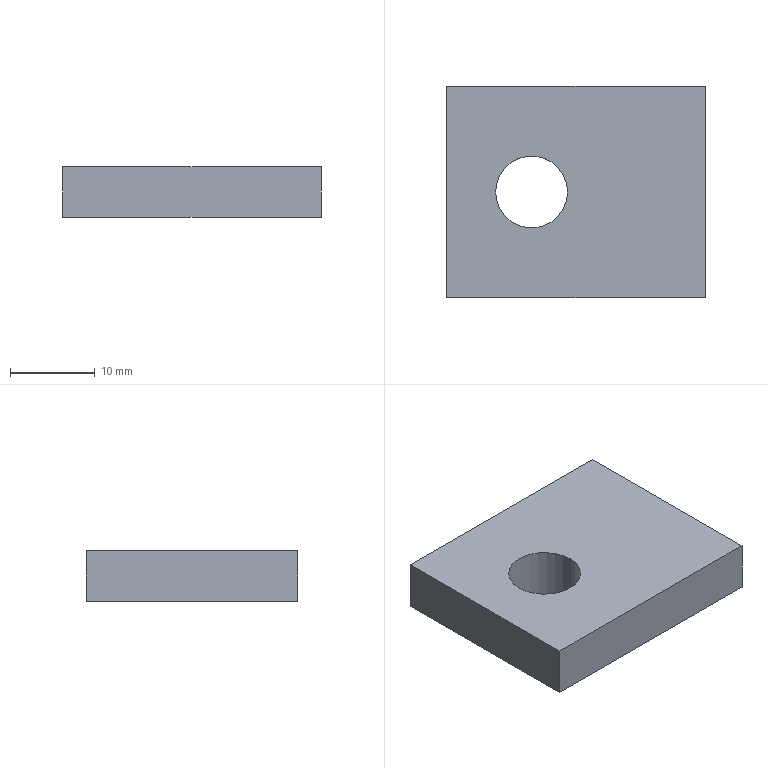Part | SolidWorks | features Extrusion 1 | 1 solid | 8 faces | box 30.5 x 25 x 6 mm | volume 4235 mm3 | plane 6 | cylinder 2 | commonest cylinder face diameters 8.5 x2
STEP:
#1=CARTESIAN_POINT('',(-30.85,-55.606,6.));
#2=VERTEX_POINT('',#1);
#3=CARTESIAN_POINT('',(-22.35,-55.606,6.));
#4=VERTEX_POINT('',#3);
#5=CARTESIAN_POINT('',(-26.6,-55.606,6.));
#6=DIRECTION('',(0.,0.,1.));
#7=DIRECTION('',(1.,0.,0.));
#8=AXIS2_PLACEMENT_3D('',#5,#6,#7);
#9=CIRCLE('',#8,4.25);
#10=EDGE_CURVE('',#2,#4,#9,.T.);
#11=ORIENTED_EDGE('',*,*,#10,.T.);
#12=CARTESIAN_POINT('',(-22.35,-55.606,0.));
#13=VERTEX_POINT('',#12);
#14=CARTESIAN_POINT('',(-22.35,-55.606,6.));
#15=DIRECTION('',(0.,0.,-1.));
#16=VECTOR('',#15,1000.);
#17=LINE('',#14,#16);
#18=EDGE_CURVE('',#4,#13,#17,.T.);
#19=ORIENTED_EDGE('',*,*,#18,.T.);
#20=CARTESIAN_POINT('',(-30.85,-55.606,0.));
#21=VERTEX_POINT('',#20);
#22=CARTESIAN_POINT('',(-26.6,-55.606,0.));
#23=DIRECTION('',(0.,0.,1.));
#24=DIRECTION('',(1.,0.,0.));
#25=AXIS2_PLACEMENT_3D('',#22,#23,#24);
#26=CIRCLE('',#25,4.25);
#27=EDGE_CURVE('',#21,#13,#26,.T.);
#28=ORIENTED_EDGE('',*,*,#27,.F.);
#29=CARTESIAN_POINT('',(-30.85,-55.606,6.));
#30=DIRECTION('',(0.,0.,-1.));
#31=VECTOR('',#30,1000.);
#32=LINE('',#29,#31);
#33=EDGE_CURVE('',#2,#21,#32,.T.);
#34=ORIENTED_EDGE('',*,*,#33,.F.);
#35=EDGE_LOOP('',(#11,#19,#28,#34));
#36=FACE_OUTER_BOUND('',#35,.T.);
#37=CARTESIAN_POINT('',(-26.6,-55.606,6.));
#38=DIRECTION('',(0.,0.,-1.));
#39=DIRECTION('',(-1.,0.,0.));
#40=AXIS2_PLACEMENT_3D('',#37,#38,#39);
#41=CYLINDRICAL_SURFACE('',#40,4.25);
#42=ADVANCED_FACE('',(#36),#41,.F.);
#43=CARTESIAN_POINT('',(-36.6,-43.106,6.));
#44=VERTEX_POINT('',#43);
#45=CARTESIAN_POINT('',(-36.6,-68.106,6.));
#46=VERTEX_POINT('',#45);
#47=CARTESIAN_POINT('',(-36.6,-43.106,6.));
#48=DIRECTION('',(0.,-1.,0.));
#49=VECTOR('',#48,1000.);
#50=LINE('',#47,#49);
#51=EDGE_CURVE('',#44,#46,#50,.T.);
#52=ORIENTED_EDGE('',*,*,#51,.T.);
#53=CARTESIAN_POINT('',(-6.1,-68.106,6.));
#54=VERTEX_POINT('',#53);
#55=CARTESIAN_POINT('',(-36.6,-68.106,6.));
#56=DIRECTION('',(1.,0.,0.));
#57=VECTOR('',#56,1000.);
#58=LINE('',#55,#57);
#59=EDGE_CURVE('',#46,#54,#58,.T.);
#60=ORIENTED_EDGE('',*,*,#59,.T.);
#61=CARTESIAN_POINT('',(-6.1,-43.106,6.));
#62=VERTEX_POINT('',#61);
#63=CARTESIAN_POINT('',(-6.1,-43.106,6.));
#64=DIRECTION('',(0.,1.,0.));
#65=VECTOR('',#64,1000.);
#66=LINE('',#63,#65);
#67=EDGE_CURVE('',#54,#62,#66,.T.);
#68=ORIENTED_EDGE('',*,*,#67,.T.);
#69=CARTESIAN_POINT('',(-36.6,-43.106,6.));
#70=DIRECTION('',(-1.,0.,0.));
#71=VECTOR('',#70,1000.);
#72=LINE('',#69,#71);
#73=EDGE_CURVE('',#62,#44,#72,.T.);
#74=ORIENTED_EDGE('',*,*,#73,.T.);
#75=EDGE_LOOP('',(#52,#60,#68,#74));
#76=FACE_OUTER_BOUND('',#75,.T.);
#77=ORIENTED_EDGE('',*,*,#10,.F.);
#78=CARTESIAN_POINT('',(-26.6,-55.606,6.));
#79=DIRECTION('',(0.,0.,1.));
#80=DIRECTION('',(1.,0.,0.));
#81=AXIS2_PLACEMENT_3D('',#78,#79,#80);
#82=CIRCLE('',#81,4.25);
#83=EDGE_CURVE('',#4,#2,#82,.T.);
#84=ORIENTED_EDGE('',*,*,#83,.F.);
#85=EDGE_LOOP('',(#77,#84));
#86=FACE_BOUND('',#85,.T.);
#87=CARTESIAN_POINT('',(0.,0.,6.));
#88=DIRECTION('',(0.,0.,1.));
#89=DIRECTION('',(1.,0.,0.));
#90=AXIS2_PLACEMENT_3D('',#87,#88,#89);
#91=PLANE('',#90);
#92=ADVANCED_FACE('',(#76,#86),#91,.T.);
#93=CARTESIAN_POINT('',(-36.6,-43.106,0.));
#94=VERTEX_POINT('',#93);
#95=CARTESIAN_POINT('',(-36.6,-68.106,0.));
#96=VERTEX_POINT('',#95);
#97=CARTESIAN_POINT('',(-36.6,-43.106,0.));
#98=DIRECTION('',(0.,-1.,0.));
#99=VECTOR('',#98,1000.);
#100=LINE('',#97,#99);
#101=EDGE_CURVE('',#94,#96,#100,.T.);
#102=ORIENTED_EDGE('',*,*,#101,.F.);
#103=CARTESIAN_POINT('',(-6.1,-43.106,0.));
#104=VERTEX_POINT('',#103);
#105=CARTESIAN_POINT('',(-36.6,-43.106,0.));
#106=DIRECTION('',(-1.,0.,0.));
#107=VECTOR('',#106,1000.);
#108=LINE('',#105,#107);
#109=EDGE_CURVE('',#104,#94,#108,.T.);
#110=ORIENTED_EDGE('',*,*,#109,.F.);
#111=CARTESIAN_POINT('',(-6.1,-68.106,0.));
#112=VERTEX_POINT('',#111);
#113=CARTESIAN_POINT('',(-6.1,-43.106,0.));
#114=DIRECTION('',(0.,1.,0.));
#115=VECTOR('',#114,1000.);
#116=LINE('',#113,#115);
#117=EDGE_CURVE('',#112,#104,#116,.T.);
#118=ORIENTED_EDGE('',*,*,#117,.F.);
#119=CARTESIAN_POINT('',(-36.6,-68.106,0.));
#120=DIRECTION('',(1.,0.,0.));
#121=VECTOR('',#120,1000.);
#122=LINE('',#119,#121);
#123=EDGE_CURVE('',#96,#112,#122,.T.);
#124=ORIENTED_EDGE('',*,*,#123,.F.);
#125=EDGE_LOOP('',(#102,#110,#118,#124));
#126=FACE_OUTER_BOUND('',#125,.T.);
#127=ORIENTED_EDGE('',*,*,#27,.T.);
#128=CARTESIAN_POINT('',(-26.6,-55.606,0.));
#129=DIRECTION('',(0.,0.,1.));
#130=DIRECTION('',(1.,0.,0.));
#131=AXIS2_PLACEMENT_3D('',#128,#129,#130);
#132=CIRCLE('',#131,4.25);
#133=EDGE_CURVE('',#13,#21,#132,.T.);
#134=ORIENTED_EDGE('',*,*,#133,.T.);
#135=EDGE_LOOP('',(#127,#134));
#136=FACE_BOUND('',#135,.T.);
#137=CARTESIAN_POINT('',(0.,0.,0.));
#138=DIRECTION('',(0.,0.,1.));
#139=DIRECTION('',(1.,0.,0.));
#140=AXIS2_PLACEMENT_3D('',#137,#138,#139);
#141=PLANE('',#140);
#142=ADVANCED_FACE('',(#126,#136),#141,.F.);
#143=ORIENTED_EDGE('',*,*,#101,.T.);
#144=CARTESIAN_POINT('',(-36.6,-68.106,6.));
#145=DIRECTION('',(0.,0.,-1.));
#146=VECTOR('',#145,1000.);
#147=LINE('',#144,#146);
#148=EDGE_CURVE('',#46,#96,#147,.T.);
#149=ORIENTED_EDGE('',*,*,#148,.F.);
#150=ORIENTED_EDGE('',*,*,#51,.F.);
#151=CARTESIAN_POINT('',(-36.6,-43.106,6.));
#152=DIRECTION('',(0.,0.,-1.));
#153=VECTOR('',#152,1000.);
#154=LINE('',#151,#153);
#155=EDGE_CURVE('',#44,#94,#154,.T.);
#156=ORIENTED_EDGE('',*,*,#155,.T.);
#157=EDGE_LOOP('',(#143,#149,#150,#156));
#158=FACE_OUTER_BOUND('',#157,.T.);
#159=CARTESIAN_POINT('',(-36.6,-43.106,6.));
#160=DIRECTION('',(1.,0.,0.));
#161=DIRECTION('',(0.,0.,-1.));
#162=AXIS2_PLACEMENT_3D('',#159,#160,#161);
#163=PLANE('',#162);
#164=ADVANCED_FACE('',(#158),#163,.F.);
#165=ORIENTED_EDGE('',*,*,#123,.T.);
#166=CARTESIAN_POINT('',(-6.1,-68.106,6.));
#167=DIRECTION('',(0.,0.,-1.));
#168=VECTOR('',#167,1000.);
#169=LINE('',#166,#168);
#170=EDGE_CURVE('',#54,#112,#169,.T.);
#171=ORIENTED_EDGE('',*,*,#170,.F.);
#172=ORIENTED_EDGE('',*,*,#59,.F.);
#173=ORIENTED_EDGE('',*,*,#148,.T.);
#174=EDGE_LOOP('',(#165,#171,#172,#173));
#175=FACE_OUTER_BOUND('',#174,.T.);
#176=CARTESIAN_POINT('',(-36.6,-68.106,6.));
#177=DIRECTION('',(0.,1.,0.));
#178=DIRECTION('',(0.,0.,1.));
#179=AXIS2_PLACEMENT_3D('',#176,#177,#178);
#180=PLANE('',#179);
#181=ADVANCED_FACE('',(#175),#180,.F.);
#182=ORIENTED_EDGE('',*,*,#117,.T.);
#183=CARTESIAN_POINT('',(-6.1,-43.106,6.));
#184=DIRECTION('',(0.,0.,-1.));
#185=VECTOR('',#184,1000.);
#186=LINE('',#183,#185);
#187=EDGE_CURVE('',#62,#104,#186,.T.);
#188=ORIENTED_EDGE('',*,*,#187,.F.);
#189=ORIENTED_EDGE('',*,*,#67,.F.);
#190=ORIENTED_EDGE('',*,*,#170,.T.);
#191=EDGE_LOOP('',(#182,#188,#189,#190));
#192=FACE_OUTER_BOUND('',#191,.T.);
#193=CARTESIAN_POINT('',(-6.1,-43.106,6.));
#194=DIRECTION('',(-1.,0.,0.));
#195=DIRECTION('',(0.,0.,1.));
#196=AXIS2_PLACEMENT_3D('',#193,#194,#195);
#197=PLANE('',#196);
#198=ADVANCED_FACE('',(#192),#197,.F.);
#199=ORIENTED_EDGE('',*,*,#109,.T.);
#200=ORIENTED_EDGE('',*,*,#155,.F.);
#201=ORIENTED_EDGE('',*,*,#73,.F.);
#202=ORIENTED_EDGE('',*,*,#187,.T.);
#203=EDGE_LOOP('',(#199,#200,#201,#202));
#204=FACE_OUTER_BOUND('',#203,.T.);
#205=CARTESIAN_POINT('',(-36.6,-43.106,6.));
#206=DIRECTION('',(0.,-1.,0.));
#207=DIRECTION('',(0.,0.,-1.));
#208=AXIS2_PLACEMENT_3D('',#205,#206,#207);
#209=PLANE('',#208);
#210=ADVANCED_FACE('',(#204),#209,.F.);
#211=ORIENTED_EDGE('',*,*,#18,.F.);
#212=ORIENTED_EDGE('',*,*,#83,.T.);
#213=ORIENTED_EDGE('',*,*,#33,.T.);
#214=ORIENTED_EDGE('',*,*,#133,.F.);
#215=EDGE_LOOP('',(#211,#212,#213,#214));
#216=FACE_OUTER_BOUND('',#215,.T.);
#217=CARTESIAN_POINT('',(-26.6,-55.606,6.));
#218=DIRECTION('',(0.,0.,-1.));
#219=DIRECTION('',(-1.,0.,0.));
#220=AXIS2_PLACEMENT_3D('',#217,#218,#219);
#221=CYLINDRICAL_SURFACE('',#220,4.25);
#222=ADVANCED_FACE('',(#216),#221,.F.);
#223=CLOSED_SHELL('',(#42,#92,#142,#164,#181,#198,#210,#222));
#224=MANIFOLD_SOLID_BREP('',#223);
#225=CARTESIAN_POINT('',(0.,0.,0.));
#226=DIRECTION('',(0.,0.,1.));
#227=DIRECTION('',(1.,0.,0.));
#228=AXIS2_PLACEMENT_3D('',#225,#226,#227);
#229=(LENGTH_UNIT()NAMED_UNIT(*)SI_UNIT(.MILLI.,.METRE.));
#230=UNCERTAINTY_MEASURE_WITH_UNIT(LENGTH_MEASURE(0.00001),#229,'','');
#231=(NAMED_UNIT(*)PLANE_ANGLE_UNIT()SI_UNIT($,.RADIAN.));
#232=(NAMED_UNIT(*)SI_UNIT($,.STERADIAN.)SOLID_ANGLE_UNIT());
#233=(GEOMETRIC_REPRESENTATION_CONTEXT(3)GLOBAL_UNCERTAINTY_ASSIGNED_CONTEXT((#230))GLOBAL_UNIT_ASSIGNED_CONTEXT((#229,#231,#232))REPRESENTATION_CONTEXT('',''));
#234=ADVANCED_BREP_SHAPE_REPRESENTATION('',(#224,#228),#233);